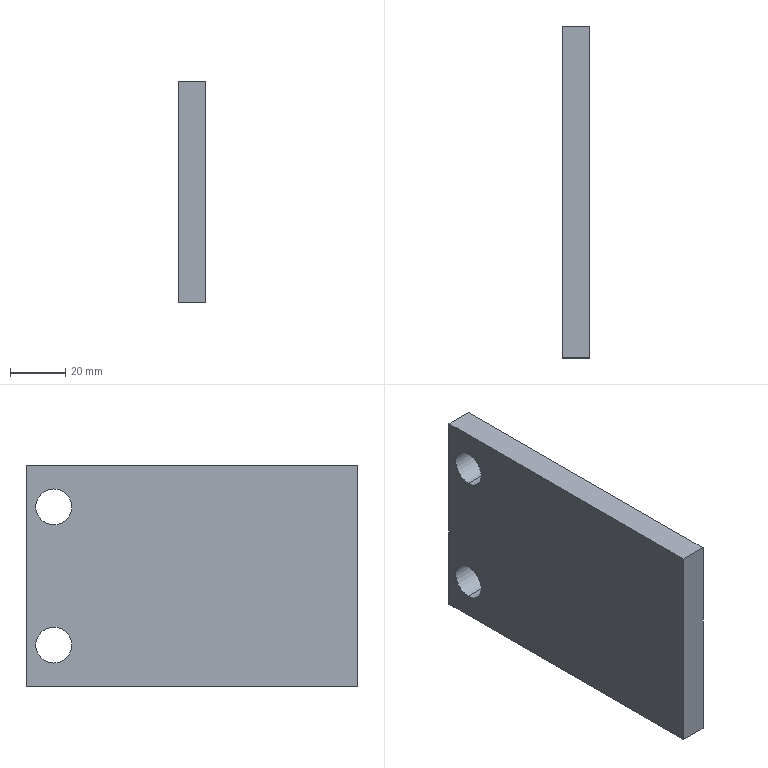Part | SolidWorks | features BaseBody 1 | 1 solid | 10 faces | box 10 x 120 x 80 mm | volume 93345 mm3 | plane 6 | cylinder 4 | commonest cylinder face diameters 13 x4
STEP:
#1=CARTESIAN_POINT('',(0.,50.,-31.5));
#2=VERTEX_POINT('',#1);
#3=CARTESIAN_POINT('',(0.,50.,-18.5));
#4=VERTEX_POINT('',#3);
#5=CARTESIAN_POINT('',(0.,50.,-25.));
#6=DIRECTION('',(-1.,0.,0.));
#7=DIRECTION('',(0.,0.,-1.));
#8=AXIS2_PLACEMENT_3D('',#5,#6,#7);
#9=CIRCLE('',#8,6.5);
#10=EDGE_CURVE('',#2,#4,#9,.T.);
#11=ORIENTED_EDGE('',*,*,#10,.T.);
#12=CARTESIAN_POINT('',(10.,50.,-18.5));
#13=VERTEX_POINT('',#12);
#14=CARTESIAN_POINT('',(-134.568,50.,-18.5));
#15=DIRECTION('',(1.,0.,0.));
#16=VECTOR('',#15,1000.);
#17=LINE('',#14,#16);
#18=EDGE_CURVE('',#4,#13,#17,.T.);
#19=ORIENTED_EDGE('',*,*,#18,.T.);
#20=CARTESIAN_POINT('',(10.,50.,-31.5));
#21=VERTEX_POINT('',#20);
#22=CARTESIAN_POINT('',(10.,50.,-25.));
#23=DIRECTION('',(-1.,0.,0.));
#24=DIRECTION('',(0.,0.,-1.));
#25=AXIS2_PLACEMENT_3D('',#22,#23,#24);
#26=CIRCLE('',#25,6.5);
#27=EDGE_CURVE('',#21,#13,#26,.T.);
#28=ORIENTED_EDGE('',*,*,#27,.F.);
#29=CARTESIAN_POINT('',(-134.568,50.,-31.5));
#30=DIRECTION('',(1.,0.,0.));
#31=VECTOR('',#30,1000.);
#32=LINE('',#29,#31);
#33=EDGE_CURVE('',#2,#21,#32,.T.);
#34=ORIENTED_EDGE('',*,*,#33,.F.);
#35=EDGE_LOOP('',(#11,#19,#28,#34));
#36=FACE_OUTER_BOUND('',#35,.T.);
#37=CARTESIAN_POINT('',(-134.568,50.,-25.));
#38=DIRECTION('',(1.,0.,0.));
#39=DIRECTION('',(0.,0.,-1.));
#40=AXIS2_PLACEMENT_3D('',#37,#38,#39);
#41=CYLINDRICAL_SURFACE('',#40,6.5);
#42=ADVANCED_FACE('',(#36),#41,.F.);
#43=CARTESIAN_POINT('',(0.,50.,18.5));
#44=VERTEX_POINT('',#43);
#45=CARTESIAN_POINT('',(0.,50.,31.5));
#46=VERTEX_POINT('',#45);
#47=CARTESIAN_POINT('',(0.,50.,25.));
#48=DIRECTION('',(-1.,0.,0.));
#49=DIRECTION('',(0.,0.,-1.));
#50=AXIS2_PLACEMENT_3D('',#47,#48,#49);
#51=CIRCLE('',#50,6.5);
#52=EDGE_CURVE('',#44,#46,#51,.T.);
#53=ORIENTED_EDGE('',*,*,#52,.T.);
#54=CARTESIAN_POINT('',(10.,50.,31.5));
#55=VERTEX_POINT('',#54);
#56=CARTESIAN_POINT('',(-134.568,50.,31.5));
#57=DIRECTION('',(1.,0.,0.));
#58=VECTOR('',#57,1000.);
#59=LINE('',#56,#58);
#60=EDGE_CURVE('',#46,#55,#59,.T.);
#61=ORIENTED_EDGE('',*,*,#60,.T.);
#62=CARTESIAN_POINT('',(10.,50.,18.5));
#63=VERTEX_POINT('',#62);
#64=CARTESIAN_POINT('',(10.,50.,25.));
#65=DIRECTION('',(-1.,0.,0.));
#66=DIRECTION('',(0.,0.,-1.));
#67=AXIS2_PLACEMENT_3D('',#64,#65,#66);
#68=CIRCLE('',#67,6.5);
#69=EDGE_CURVE('',#63,#55,#68,.T.);
#70=ORIENTED_EDGE('',*,*,#69,.F.);
#71=CARTESIAN_POINT('',(-134.568,50.,18.5));
#72=DIRECTION('',(1.,0.,0.));
#73=VECTOR('',#72,1000.);
#74=LINE('',#71,#73);
#75=EDGE_CURVE('',#44,#63,#74,.T.);
#76=ORIENTED_EDGE('',*,*,#75,.F.);
#77=EDGE_LOOP('',(#53,#61,#70,#76));
#78=FACE_OUTER_BOUND('',#77,.T.);
#79=CARTESIAN_POINT('',(-134.568,50.,25.));
#80=DIRECTION('',(1.,0.,0.));
#81=DIRECTION('',(0.,0.,-1.));
#82=AXIS2_PLACEMENT_3D('',#79,#80,#81);
#83=CYLINDRICAL_SURFACE('',#82,6.5);
#84=ADVANCED_FACE('',(#78),#83,.F.);
#85=ORIENTED_EDGE('',*,*,#10,.F.);
#86=CARTESIAN_POINT('',(0.,50.,-25.));
#87=DIRECTION('',(-1.,0.,0.));
#88=DIRECTION('',(0.,0.,-1.));
#89=AXIS2_PLACEMENT_3D('',#86,#87,#88);
#90=CIRCLE('',#89,6.5);
#91=EDGE_CURVE('',#4,#2,#90,.T.);
#92=ORIENTED_EDGE('',*,*,#91,.F.);
#93=EDGE_LOOP('',(#85,#92));
#94=FACE_BOUND('',#93,.T.);
#95=ORIENTED_EDGE('',*,*,#52,.F.);
#96=CARTESIAN_POINT('',(0.,50.,25.));
#97=DIRECTION('',(-1.,0.,0.));
#98=DIRECTION('',(0.,0.,-1.));
#99=AXIS2_PLACEMENT_3D('',#96,#97,#98);
#100=CIRCLE('',#99,6.5);
#101=EDGE_CURVE('',#46,#44,#100,.T.);
#102=ORIENTED_EDGE('',*,*,#101,.F.);
#103=EDGE_LOOP('',(#95,#102));
#104=FACE_BOUND('',#103,.T.);
#105=CARTESIAN_POINT('',(0.,60.,-40.));
#106=VERTEX_POINT('',#105);
#107=CARTESIAN_POINT('',(0.,60.,40.));
#108=VERTEX_POINT('',#107);
#109=CARTESIAN_POINT('',(0.,60.,0.));
#110=DIRECTION('',(0.,0.,1.));
#111=VECTOR('',#110,1000.);
#112=LINE('',#109,#111);
#113=EDGE_CURVE('',#106,#108,#112,.T.);
#114=ORIENTED_EDGE('',*,*,#113,.F.);
#115=CARTESIAN_POINT('',(0.,-60.,-40.));
#116=VERTEX_POINT('',#115);
#117=CARTESIAN_POINT('',(0.,0.,-40.));
#118=DIRECTION('',(0.,1.,0.));
#119=VECTOR('',#118,1000.);
#120=LINE('',#117,#119);
#121=EDGE_CURVE('',#116,#106,#120,.T.);
#122=ORIENTED_EDGE('',*,*,#121,.F.);
#123=CARTESIAN_POINT('',(0.,-60.,40.));
#124=VERTEX_POINT('',#123);
#125=CARTESIAN_POINT('',(0.,-60.,0.));
#126=DIRECTION('',(0.,0.,-1.));
#127=VECTOR('',#126,1000.);
#128=LINE('',#125,#127);
#129=EDGE_CURVE('',#124,#116,#128,.T.);
#130=ORIENTED_EDGE('',*,*,#129,.F.);
#131=CARTESIAN_POINT('',(0.,0.,40.));
#132=DIRECTION('',(0.,-1.,0.));
#133=VECTOR('',#132,1000.);
#134=LINE('',#131,#133);
#135=EDGE_CURVE('',#108,#124,#134,.T.);
#136=ORIENTED_EDGE('',*,*,#135,.F.);
#137=EDGE_LOOP('',(#114,#122,#130,#136));
#138=FACE_OUTER_BOUND('',#137,.T.);
#139=CARTESIAN_POINT('',(0.,0.,0.));
#140=DIRECTION('',(1.,0.,0.));
#141=DIRECTION('',(0.,0.,-1.));
#142=AXIS2_PLACEMENT_3D('',#139,#140,#141);
#143=PLANE('',#142);
#144=ADVANCED_FACE('',(#94,#104,#138),#143,.F.);
#145=ORIENTED_EDGE('',*,*,#18,.F.);
#146=ORIENTED_EDGE('',*,*,#91,.T.);
#147=ORIENTED_EDGE('',*,*,#33,.T.);
#148=CARTESIAN_POINT('',(10.,50.,-25.));
#149=DIRECTION('',(-1.,0.,0.));
#150=DIRECTION('',(0.,0.,-1.));
#151=AXIS2_PLACEMENT_3D('',#148,#149,#150);
#152=CIRCLE('',#151,6.5);
#153=EDGE_CURVE('',#13,#21,#152,.T.);
#154=ORIENTED_EDGE('',*,*,#153,.F.);
#155=EDGE_LOOP('',(#145,#146,#147,#154));
#156=FACE_OUTER_BOUND('',#155,.T.);
#157=CARTESIAN_POINT('',(-134.568,50.,-25.));
#158=DIRECTION('',(1.,0.,0.));
#159=DIRECTION('',(0.,0.,-1.));
#160=AXIS2_PLACEMENT_3D('',#157,#158,#159);
#161=CYLINDRICAL_SURFACE('',#160,6.5);
#162=ADVANCED_FACE('',(#156),#161,.F.);
#163=ORIENTED_EDGE('',*,*,#60,.F.);
#164=ORIENTED_EDGE('',*,*,#101,.T.);
#165=ORIENTED_EDGE('',*,*,#75,.T.);
#166=CARTESIAN_POINT('',(10.,50.,25.));
#167=DIRECTION('',(-1.,0.,0.));
#168=DIRECTION('',(0.,0.,-1.));
#169=AXIS2_PLACEMENT_3D('',#166,#167,#168);
#170=CIRCLE('',#169,6.5);
#171=EDGE_CURVE('',#55,#63,#170,.T.);
#172=ORIENTED_EDGE('',*,*,#171,.F.);
#173=EDGE_LOOP('',(#163,#164,#165,#172));
#174=FACE_OUTER_BOUND('',#173,.T.);
#175=CARTESIAN_POINT('',(-134.568,50.,25.));
#176=DIRECTION('',(1.,0.,0.));
#177=DIRECTION('',(0.,0.,-1.));
#178=AXIS2_PLACEMENT_3D('',#175,#176,#177);
#179=CYLINDRICAL_SURFACE('',#178,6.5);
#180=ADVANCED_FACE('',(#174),#179,.F.);
#181=CARTESIAN_POINT('',(10.,-60.,40.));
#182=VERTEX_POINT('',#181);
#183=CARTESIAN_POINT('',(10.,60.,40.));
#184=VERTEX_POINT('',#183);
#185=CARTESIAN_POINT('',(10.,60.,40.));
#186=DIRECTION('',(0.,1.,0.));
#187=VECTOR('',#186,1000.);
#188=LINE('',#185,#187);
#189=EDGE_CURVE('',#182,#184,#188,.T.);
#190=ORIENTED_EDGE('',*,*,#189,.T.);
#191=CARTESIAN_POINT('',(0.,60.,40.));
#192=DIRECTION('',(-1.,0.,0.));
#193=VECTOR('',#192,1000.);
#194=LINE('',#191,#193);
#195=EDGE_CURVE('',#184,#108,#194,.T.);
#196=ORIENTED_EDGE('',*,*,#195,.T.);
#197=ORIENTED_EDGE('',*,*,#135,.T.);
#198=CARTESIAN_POINT('',(0.,-60.,40.));
#199=DIRECTION('',(1.,0.,0.));
#200=VECTOR('',#199,1000.);
#201=LINE('',#198,#200);
#202=EDGE_CURVE('',#124,#182,#201,.T.);
#203=ORIENTED_EDGE('',*,*,#202,.T.);
#204=EDGE_LOOP('',(#190,#196,#197,#203));
#205=FACE_OUTER_BOUND('',#204,.T.);
#206=CARTESIAN_POINT('',(0.,60.,40.));
#207=DIRECTION('',(0.,0.,1.));
#208=DIRECTION('',(1.,0.,0.));
#209=AXIS2_PLACEMENT_3D('',#206,#207,#208);
#210=PLANE('',#209);
#211=ADVANCED_FACE('',(#205),#210,.T.);
#212=CARTESIAN_POINT('',(10.,60.,-40.));
#213=VERTEX_POINT('',#212);
#214=CARTESIAN_POINT('',(10.,60.,-40.));
#215=DIRECTION('',(0.,0.,-1.));
#216=VECTOR('',#215,1000.);
#217=LINE('',#214,#216);
#218=EDGE_CURVE('',#184,#213,#217,.T.);
#219=ORIENTED_EDGE('',*,*,#218,.T.);
#220=CARTESIAN_POINT('',(0.,60.,-40.));
#221=DIRECTION('',(-1.,0.,0.));
#222=VECTOR('',#221,1000.);
#223=LINE('',#220,#222);
#224=EDGE_CURVE('',#213,#106,#223,.T.);
#225=ORIENTED_EDGE('',*,*,#224,.T.);
#226=ORIENTED_EDGE('',*,*,#113,.T.);
#227=ORIENTED_EDGE('',*,*,#195,.F.);
#228=EDGE_LOOP('',(#219,#225,#226,#227));
#229=FACE_OUTER_BOUND('',#228,.T.);
#230=CARTESIAN_POINT('',(0.,60.,-40.));
#231=DIRECTION('',(0.,1.,0.));
#232=DIRECTION('',(0.,0.,1.));
#233=AXIS2_PLACEMENT_3D('',#230,#231,#232);
#234=PLANE('',#233);
#235=ADVANCED_FACE('',(#229),#234,.T.);
#236=CARTESIAN_POINT('',(10.,-60.,-40.));
#237=VERTEX_POINT('',#236);
#238=CARTESIAN_POINT('',(10.,-60.,-40.));
#239=DIRECTION('',(0.,-1.,0.));
#240=VECTOR('',#239,1000.);
#241=LINE('',#238,#240);
#242=EDGE_CURVE('',#213,#237,#241,.T.);
#243=ORIENTED_EDGE('',*,*,#242,.T.);
#244=CARTESIAN_POINT('',(0.,-60.,-40.));
#245=DIRECTION('',(-1.,0.,0.));
#246=VECTOR('',#245,1000.);
#247=LINE('',#244,#246);
#248=EDGE_CURVE('',#237,#116,#247,.T.);
#249=ORIENTED_EDGE('',*,*,#248,.T.);
#250=ORIENTED_EDGE('',*,*,#121,.T.);
#251=ORIENTED_EDGE('',*,*,#224,.F.);
#252=EDGE_LOOP('',(#243,#249,#250,#251));
#253=FACE_OUTER_BOUND('',#252,.T.);
#254=CARTESIAN_POINT('',(0.,-60.,-40.));
#255=DIRECTION('',(0.,0.,-1.));
#256=DIRECTION('',(0.,1.,0.));
#257=AXIS2_PLACEMENT_3D('',#254,#255,#256);
#258=PLANE('',#257);
#259=ADVANCED_FACE('',(#253),#258,.T.);
#260=CARTESIAN_POINT('',(10.,-60.,40.));
#261=DIRECTION('',(0.,0.,1.));
#262=VECTOR('',#261,1000.);
#263=LINE('',#260,#262);
#264=EDGE_CURVE('',#237,#182,#263,.T.);
#265=ORIENTED_EDGE('',*,*,#264,.T.);
#266=ORIENTED_EDGE('',*,*,#202,.F.);
#267=ORIENTED_EDGE('',*,*,#129,.T.);
#268=ORIENTED_EDGE('',*,*,#248,.F.);
#269=EDGE_LOOP('',(#265,#266,#267,#268));
#270=FACE_OUTER_BOUND('',#269,.T.);
#271=CARTESIAN_POINT('',(0.,-60.,40.));
#272=DIRECTION('',(0.,-1.,0.));
#273=DIRECTION('',(0.,0.,-1.));
#274=AXIS2_PLACEMENT_3D('',#271,#272,#273);
#275=PLANE('',#274);
#276=ADVANCED_FACE('',(#270),#275,.T.);
#277=ORIENTED_EDGE('',*,*,#27,.T.);
#278=ORIENTED_EDGE('',*,*,#153,.T.);
#279=EDGE_LOOP('',(#277,#278));
#280=FACE_BOUND('',#279,.T.);
#281=ORIENTED_EDGE('',*,*,#69,.T.);
#282=ORIENTED_EDGE('',*,*,#171,.T.);
#283=EDGE_LOOP('',(#281,#282));
#284=FACE_BOUND('',#283,.T.);
#285=ORIENTED_EDGE('',*,*,#242,.F.);
#286=ORIENTED_EDGE('',*,*,#218,.F.);
#287=ORIENTED_EDGE('',*,*,#189,.F.);
#288=ORIENTED_EDGE('',*,*,#264,.F.);
#289=EDGE_LOOP('',(#285,#286,#287,#288));
#290=FACE_OUTER_BOUND('',#289,.T.);
#291=CARTESIAN_POINT('',(10.,0.,0.));
#292=DIRECTION('',(1.,0.,0.));
#293=DIRECTION('',(0.,0.,-1.));
#294=AXIS2_PLACEMENT_3D('',#291,#292,#293);
#295=PLANE('',#294);
#296=ADVANCED_FACE('',(#280,#284,#290),#295,.T.);
#297=CLOSED_SHELL('',(#42,#84,#144,#162,#180,#211,#235,#259,#276,#296));
#298=MANIFOLD_SOLID_BREP('',#297);
#299=CARTESIAN_POINT('',(0.,0.,0.));
#300=DIRECTION('',(0.,0.,1.));
#301=DIRECTION('',(1.,0.,0.));
#302=AXIS2_PLACEMENT_3D('',#299,#300,#301);
#303=(LENGTH_UNIT()NAMED_UNIT(*)SI_UNIT(.MILLI.,.METRE.));
#304=UNCERTAINTY_MEASURE_WITH_UNIT(LENGTH_MEASURE(0.00001),#303,'','');
#305=(NAMED_UNIT(*)PLANE_ANGLE_UNIT()SI_UNIT($,.RADIAN.));
#306=(NAMED_UNIT(*)SI_UNIT($,.STERADIAN.)SOLID_ANGLE_UNIT());
#307=(GEOMETRIC_REPRESENTATION_CONTEXT(3)GLOBAL_UNCERTAINTY_ASSIGNED_CONTEXT((#304))GLOBAL_UNIT_ASSIGNED_CONTEXT((#303,#305,#306))REPRESENTATION_CONTEXT('',''));
#308=ADVANCED_BREP_SHAPE_REPRESENTATION('',(#298,#302),#307);